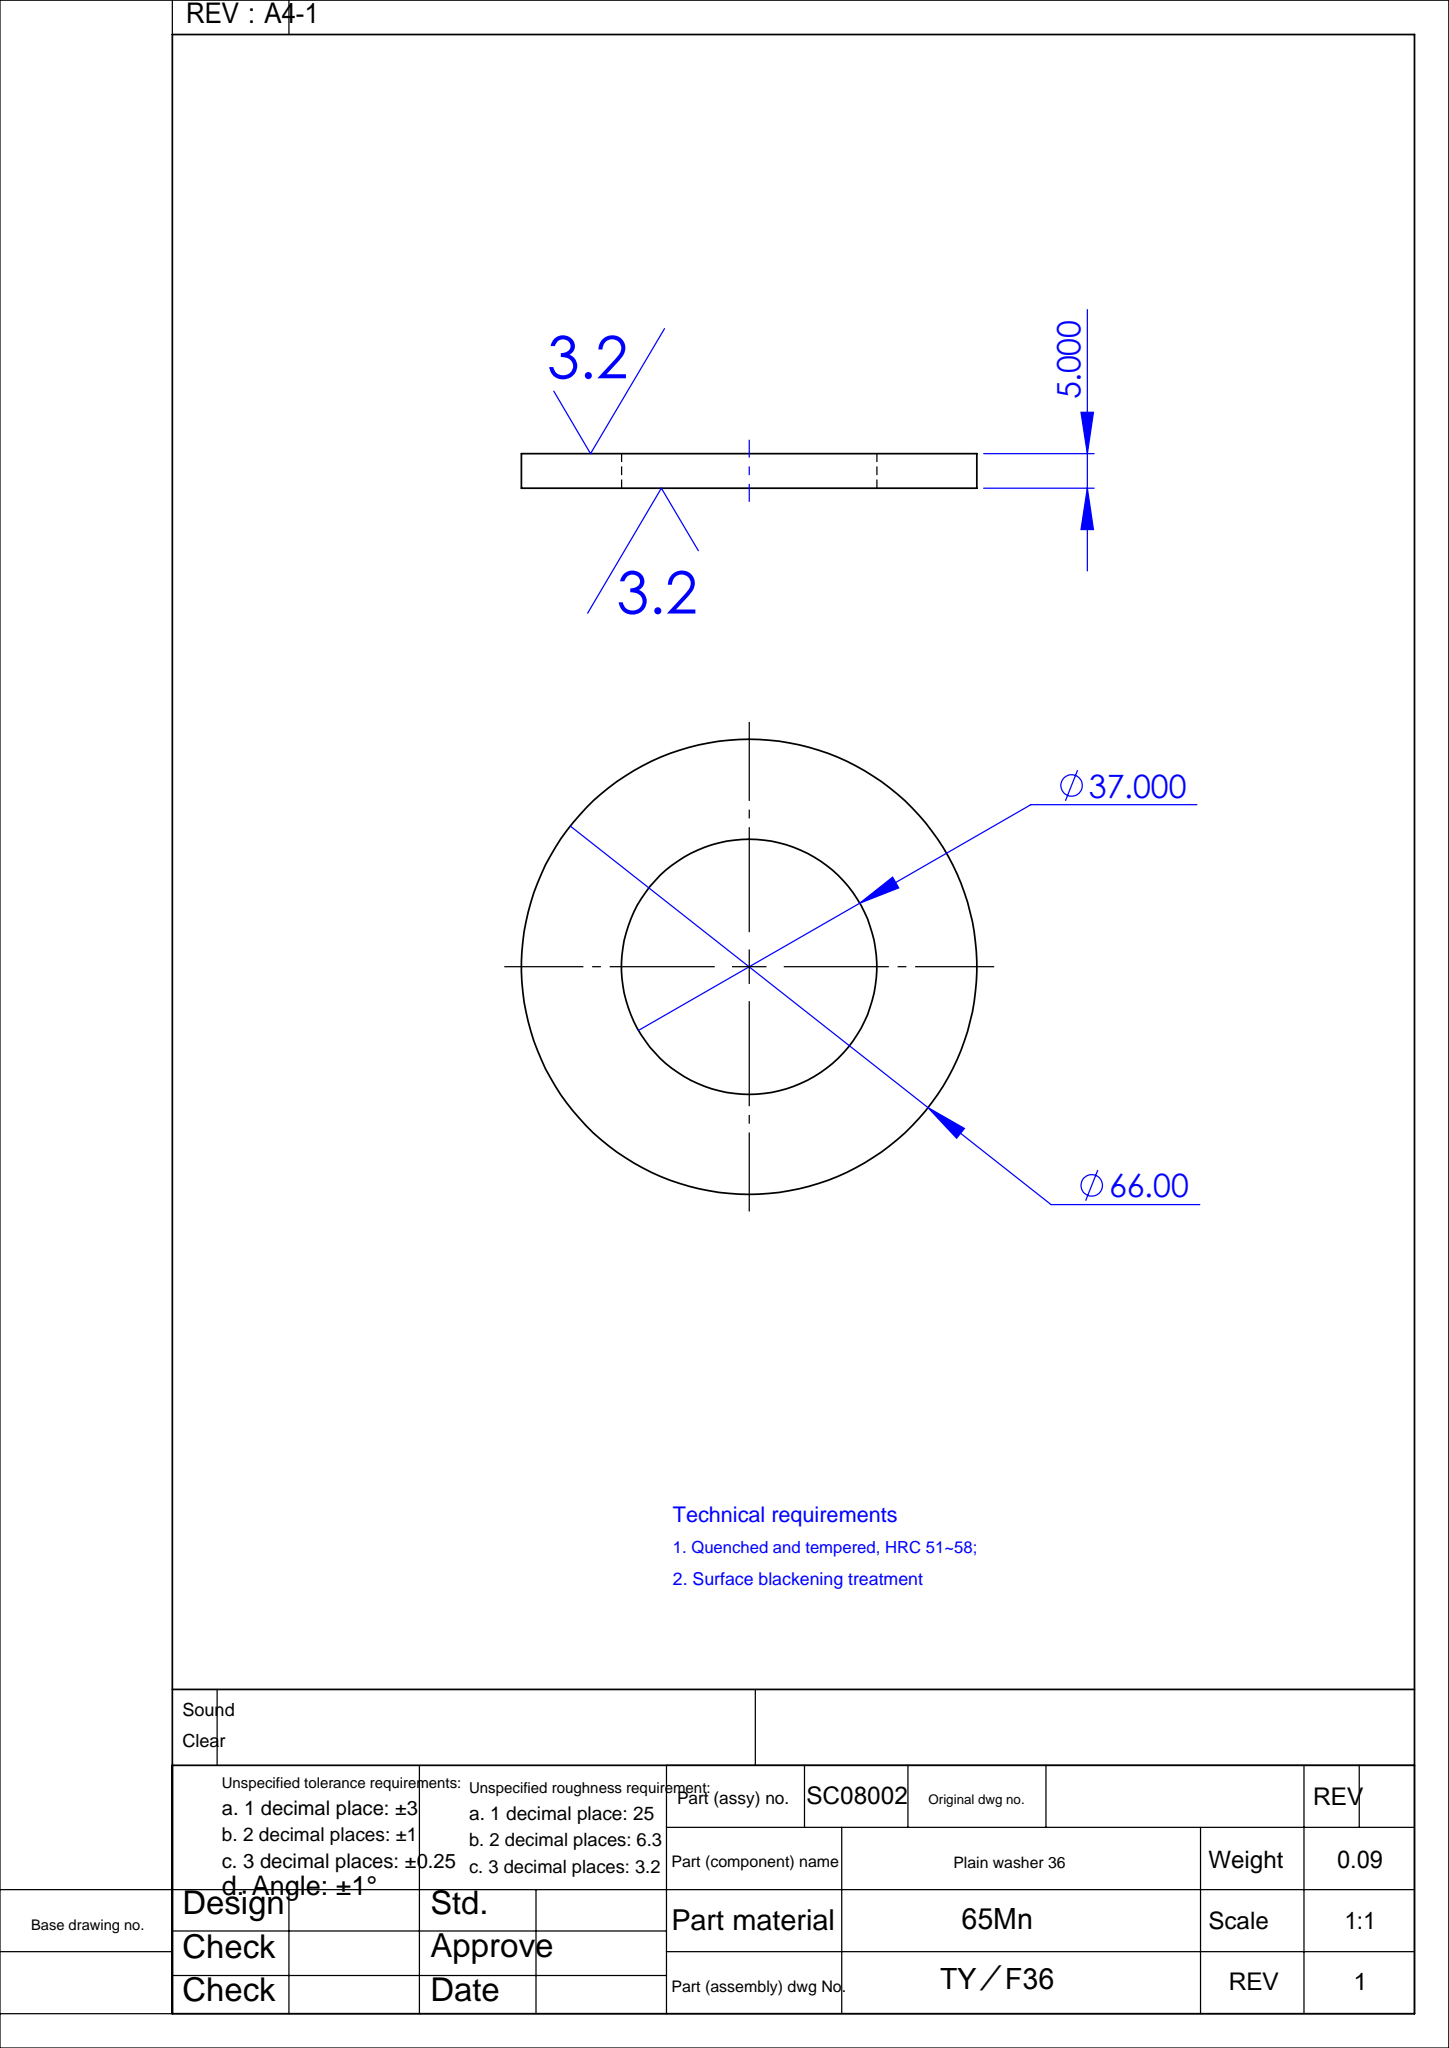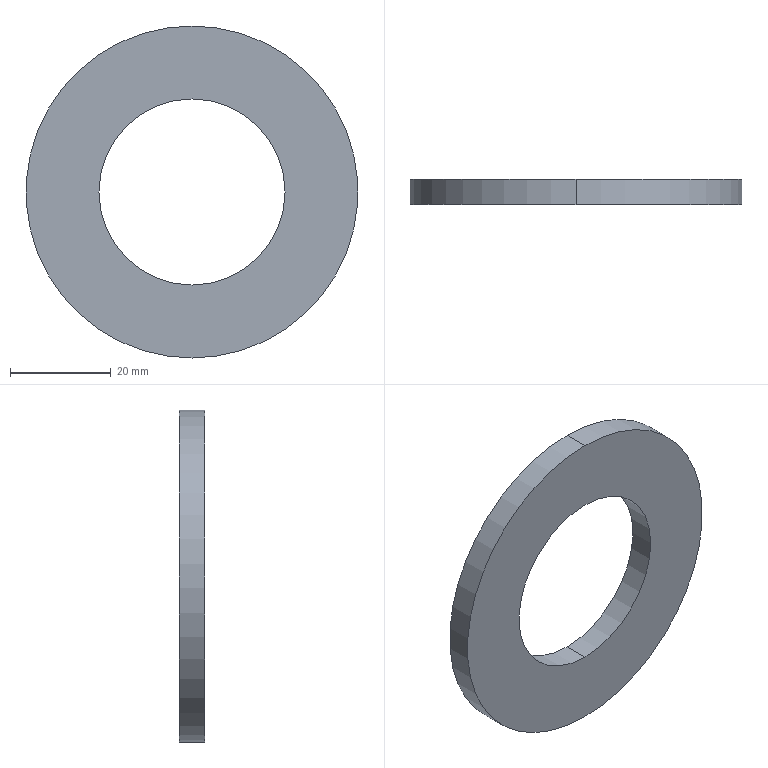Part | SolidWorks | features Revolution 1 | 1 solid | 6 faces | box 66 x 5 x 66 mm | volume 11730 mm3 | cylinder 4 | plane 2 | commonest cylinder face diameters 37 x2 66 x2
STEP:
#1=CARTESIAN_POINT('',(0.,13.645,-33.));
#2=VERTEX_POINT('',#1);
#3=CARTESIAN_POINT('',(0.,13.645,33.));
#4=VERTEX_POINT('',#3);
#5=CARTESIAN_POINT('',(0.,13.645,0.));
#6=DIRECTION('',(0.,-1.,0.));
#7=DIRECTION('',(0.,0.,-1.));
#8=AXIS2_PLACEMENT_3D('',#5,#6,#7);
#9=CIRCLE('',#8,33.);
#10=EDGE_CURVE('',#2,#4,#9,.T.);
#11=ORIENTED_EDGE('',*,*,#10,.T.);
#12=CARTESIAN_POINT('',(0.,8.645,33.));
#13=VERTEX_POINT('',#12);
#14=CARTESIAN_POINT('',(0.,0.,33.));
#15=DIRECTION('',(0.,-1.,0.));
#16=VECTOR('',#15,1000.);
#17=LINE('',#14,#16);
#18=EDGE_CURVE('',#4,#13,#17,.T.);
#19=ORIENTED_EDGE('',*,*,#18,.T.);
#20=CARTESIAN_POINT('',(0.,8.645,-33.));
#21=VERTEX_POINT('',#20);
#22=CARTESIAN_POINT('',(0.,8.645,0.));
#23=DIRECTION('',(0.,-1.,0.));
#24=DIRECTION('',(0.,0.,-1.));
#25=AXIS2_PLACEMENT_3D('',#22,#23,#24);
#26=CIRCLE('',#25,33.);
#27=EDGE_CURVE('',#21,#13,#26,.T.);
#28=ORIENTED_EDGE('',*,*,#27,.F.);
#29=CARTESIAN_POINT('',(0.,0.,-33.));
#30=DIRECTION('',(0.,-1.,0.));
#31=VECTOR('',#30,1000.);
#32=LINE('',#29,#31);
#33=EDGE_CURVE('',#2,#21,#32,.T.);
#34=ORIENTED_EDGE('',*,*,#33,.F.);
#35=EDGE_LOOP('',(#11,#19,#28,#34));
#36=FACE_OUTER_BOUND('',#35,.T.);
#37=CARTESIAN_POINT('',(0.,0.,0.));
#38=DIRECTION('',(0.,-1.,0.));
#39=DIRECTION('',(0.,0.,-1.));
#40=AXIS2_PLACEMENT_3D('',#37,#38,#39);
#41=CYLINDRICAL_SURFACE('',#40,33.);
#42=ADVANCED_FACE('',(#36),#41,.T.);
#43=CARTESIAN_POINT('',(0.,13.645,18.5));
#44=VERTEX_POINT('',#43);
#45=CARTESIAN_POINT('',(0.,13.645,-18.5));
#46=VERTEX_POINT('',#45);
#47=CARTESIAN_POINT('',(0.,13.645,0.));
#48=DIRECTION('',(0.,-1.,0.));
#49=DIRECTION('',(0.,0.,-1.));
#50=AXIS2_PLACEMENT_3D('',#47,#48,#49);
#51=CIRCLE('',#50,18.5);
#52=EDGE_CURVE('',#44,#46,#51,.T.);
#53=ORIENTED_EDGE('',*,*,#52,.F.);
#54=CARTESIAN_POINT('',(0.,8.645,18.5));
#55=VERTEX_POINT('',#54);
#56=CARTESIAN_POINT('',(0.,0.,18.5));
#57=DIRECTION('',(0.,-1.,0.));
#58=VECTOR('',#57,1000.);
#59=LINE('',#56,#58);
#60=EDGE_CURVE('',#44,#55,#59,.T.);
#61=ORIENTED_EDGE('',*,*,#60,.T.);
#62=CARTESIAN_POINT('',(0.,8.645,-18.5));
#63=VERTEX_POINT('',#62);
#64=CARTESIAN_POINT('',(0.,8.645,0.));
#65=DIRECTION('',(0.,-1.,0.));
#66=DIRECTION('',(0.,0.,-1.));
#67=AXIS2_PLACEMENT_3D('',#64,#65,#66);
#68=CIRCLE('',#67,18.5);
#69=EDGE_CURVE('',#55,#63,#68,.T.);
#70=ORIENTED_EDGE('',*,*,#69,.T.);
#71=CARTESIAN_POINT('',(0.,0.,-18.5));
#72=DIRECTION('',(0.,-1.,0.));
#73=VECTOR('',#72,1000.);
#74=LINE('',#71,#73);
#75=EDGE_CURVE('',#46,#63,#74,.T.);
#76=ORIENTED_EDGE('',*,*,#75,.F.);
#77=EDGE_LOOP('',(#53,#61,#70,#76));
#78=FACE_OUTER_BOUND('',#77,.T.);
#79=CARTESIAN_POINT('',(0.,0.,0.));
#80=DIRECTION('',(0.,-1.,0.));
#81=DIRECTION('',(0.,0.,-1.));
#82=AXIS2_PLACEMENT_3D('',#79,#80,#81);
#83=CYLINDRICAL_SURFACE('',#82,18.5);
#84=ADVANCED_FACE('',(#78),#83,.F.);
#85=ORIENTED_EDGE('',*,*,#60,.F.);
#86=CARTESIAN_POINT('',(0.,13.645,0.));
#87=DIRECTION('',(0.,-1.,0.));
#88=DIRECTION('',(0.,0.,-1.));
#89=AXIS2_PLACEMENT_3D('',#86,#87,#88);
#90=CIRCLE('',#89,18.5);
#91=EDGE_CURVE('',#46,#44,#90,.T.);
#92=ORIENTED_EDGE('',*,*,#91,.F.);
#93=ORIENTED_EDGE('',*,*,#75,.T.);
#94=CARTESIAN_POINT('',(0.,8.645,0.));
#95=DIRECTION('',(0.,-1.,0.));
#96=DIRECTION('',(0.,0.,-1.));
#97=AXIS2_PLACEMENT_3D('',#94,#95,#96);
#98=CIRCLE('',#97,18.5);
#99=EDGE_CURVE('',#63,#55,#98,.T.);
#100=ORIENTED_EDGE('',*,*,#99,.T.);
#101=EDGE_LOOP('',(#85,#92,#93,#100));
#102=FACE_OUTER_BOUND('',#101,.T.);
#103=CARTESIAN_POINT('',(0.,0.,0.));
#104=DIRECTION('',(0.,-1.,0.));
#105=DIRECTION('',(0.,0.,-1.));
#106=AXIS2_PLACEMENT_3D('',#103,#104,#105);
#107=CYLINDRICAL_SURFACE('',#106,18.5);
#108=ADVANCED_FACE('',(#102),#107,.F.);
#109=ORIENTED_EDGE('',*,*,#10,.F.);
#110=CARTESIAN_POINT('',(0.,13.645,0.));
#111=DIRECTION('',(0.,-1.,0.));
#112=DIRECTION('',(0.,0.,-1.));
#113=AXIS2_PLACEMENT_3D('',#110,#111,#112);
#114=CIRCLE('',#113,33.);
#115=EDGE_CURVE('',#4,#2,#114,.T.);
#116=ORIENTED_EDGE('',*,*,#115,.F.);
#117=EDGE_LOOP('',(#109,#116));
#118=FACE_OUTER_BOUND('',#117,.T.);
#119=ORIENTED_EDGE('',*,*,#91,.T.);
#120=ORIENTED_EDGE('',*,*,#52,.T.);
#121=EDGE_LOOP('',(#119,#120));
#122=FACE_BOUND('',#121,.T.);
#123=CARTESIAN_POINT('',(-18.5,13.645,0.));
#124=DIRECTION('',(0.,-1.,0.));
#125=DIRECTION('',(0.,0.,-1.));
#126=AXIS2_PLACEMENT_3D('',#123,#124,#125);
#127=PLANE('',#126);
#128=ADVANCED_FACE('',(#118,#122),#127,.F.);
#129=ORIENTED_EDGE('',*,*,#18,.F.);
#130=ORIENTED_EDGE('',*,*,#115,.T.);
#131=ORIENTED_EDGE('',*,*,#33,.T.);
#132=CARTESIAN_POINT('',(0.,8.645,0.));
#133=DIRECTION('',(0.,-1.,0.));
#134=DIRECTION('',(0.,0.,-1.));
#135=AXIS2_PLACEMENT_3D('',#132,#133,#134);
#136=CIRCLE('',#135,33.);
#137=EDGE_CURVE('',#13,#21,#136,.T.);
#138=ORIENTED_EDGE('',*,*,#137,.F.);
#139=EDGE_LOOP('',(#129,#130,#131,#138));
#140=FACE_OUTER_BOUND('',#139,.T.);
#141=CARTESIAN_POINT('',(0.,0.,0.));
#142=DIRECTION('',(0.,-1.,0.));
#143=DIRECTION('',(0.,0.,-1.));
#144=AXIS2_PLACEMENT_3D('',#141,#142,#143);
#145=CYLINDRICAL_SURFACE('',#144,33.);
#146=ADVANCED_FACE('',(#140),#145,.T.);
#147=ORIENTED_EDGE('',*,*,#99,.F.);
#148=ORIENTED_EDGE('',*,*,#69,.F.);
#149=EDGE_LOOP('',(#147,#148));
#150=FACE_BOUND('',#149,.T.);
#151=ORIENTED_EDGE('',*,*,#27,.T.);
#152=ORIENTED_EDGE('',*,*,#137,.T.);
#153=EDGE_LOOP('',(#151,#152));
#154=FACE_OUTER_BOUND('',#153,.T.);
#155=CARTESIAN_POINT('',(-18.5,8.645,0.));
#156=DIRECTION('',(0.,1.,0.));
#157=DIRECTION('',(0.,0.,1.));
#158=AXIS2_PLACEMENT_3D('',#155,#156,#157);
#159=PLANE('',#158);
#160=ADVANCED_FACE('',(#150,#154),#159,.F.);
#161=CLOSED_SHELL('',(#42,#84,#108,#128,#146,#160));
#162=MANIFOLD_SOLID_BREP('',#161);
#163=CARTESIAN_POINT('',(0.,0.,0.));
#164=DIRECTION('',(0.,0.,1.));
#165=DIRECTION('',(1.,0.,0.));
#166=AXIS2_PLACEMENT_3D('',#163,#164,#165);
#167=(LENGTH_UNIT()NAMED_UNIT(*)SI_UNIT(.MILLI.,.METRE.));
#168=UNCERTAINTY_MEASURE_WITH_UNIT(LENGTH_MEASURE(0.00001),#167,'','');
#169=(NAMED_UNIT(*)PLANE_ANGLE_UNIT()SI_UNIT($,.RADIAN.));
#170=(NAMED_UNIT(*)SI_UNIT($,.STERADIAN.)SOLID_ANGLE_UNIT());
#171=(GEOMETRIC_REPRESENTATION_CONTEXT(3)GLOBAL_UNCERTAINTY_ASSIGNED_CONTEXT((#168))GLOBAL_UNIT_ASSIGNED_CONTEXT((#167,#169,#170))REPRESENTATION_CONTEXT('',''));
#172=ADVANCED_BREP_SHAPE_REPRESENTATION('',(#162,#166),#171);